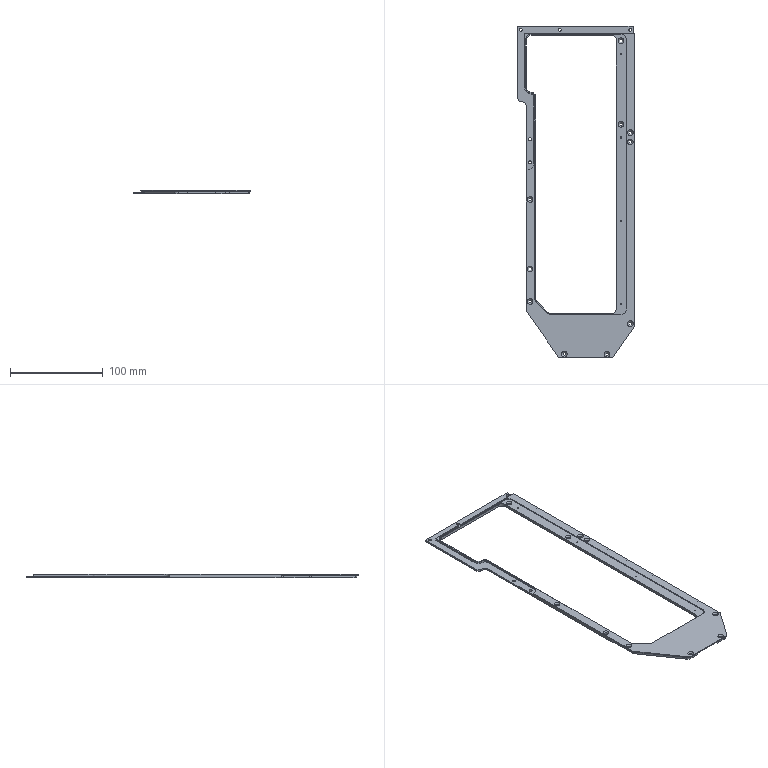NC program | NX | posted with a generic post | part box 127 x 358 x 4 mm
Whole program:
N10 G17 G21 G94 G90
(SPOT_DRILL , TOOL : CHAMFER_D8-90DEG)
N12 T01 M6
N14 G53
N16 G17 G0 G90 X153.952 Y-40.61 S2500 M3
N18 G43 Z20. H1
N20 G94 G82 G98 Z-2.6 F250. P200 R3.
N22 X103.952 Y-30.61
N24 X48.952
N26 X-6.048
N28 X-61.048
N30 X-111.048
N32 X-101. Y3.5
N34 X-111.048 Y28.911
N36 X-61.048
N38 X-6.048
N40 X48.952
N42 X103.952
N44 X119. Y3.5
N46 X153.952 Y28.911
N48 G80
N50 G0 X153.952 Y28.911 Z20.
N52 M5
(SPOT_DRILL_COPY , TOOL : DRILL_D5.3-62-92)
N54 T02 M6
N56 G53
N58 G17 G0 G90 X153.952 Y-40.61 S3000 M3
N60 G43 Z20. H2
N62 G94 G82 G98 Z-6.5 F200. P200 R3.
N64 X103.952 Y-30.61
N66 X48.952
N68 X-6.048
N70 X-61.048
N72 X-111.048
N74 X-101. Y3.5
N76 X-111.048 Y28.911
N78 X-61.048
N80 X-6.048
N82 X48.952
N84 X103.952
N86 X119. Y3.5
N88 X153.952 Y28.911
N90 G80
N92 G0 X153.952 Y28.911 Z20.
N94 M5
(SPOT_DRILL_1 , TOOL : CHAMFER_D8-90DEG)
N96 T01 M6
N98 G53
N100 G17 G0 G90 X175. Y-59.5 S2500 M3
N102 G43 Z20. H1
N104 G94 G82 G98 Z-1.6 F250. P200 R3.
N106 Y-17.5
N108 Y58.5
N110 X163. Y48.5
N112 X73.
N114 X64. Y58.5
N116 X54.
N118 X57. Y-49.5
N120 X32.
N122 X-8.
N124 X-83.
N126 X-118.
N128 X-175. Y-12.5
N130 Y33.5
N132 X-142. Y58.5
N134 G80
N136 G0 X-142. Y58.5 Z20.
N138 M5
(SPOT_DRILL_1_COPY , TOOL : DRILL_D3.2-42-71)
N140 T06 M6
N142 G53
N144 G17 G0 G90 X175. Y-59.5 S3000 M3
N146 G43 Z20. H6
N148 G94 G82 G98 Z-6. F200. P200 R3.
N150 Y-17.5
N152 Y58.5
N154 X163. Y48.5
N156 X73.
N158 X64. Y58.5
N160 X54.
N162 X57. Y-49.5
N164 X32.
N166 X-8.
N168 X-83.
N170 X-118.
N172 X-175. Y-12.5
N174 Y33.5
N176 X-142. Y58.5
N178 G80
N180 G0 X-142. Y58.5 Z20.
N182 M5
(PLANAR_MILL_9 , TOOL : D6-18-D6-50-3T-ROUGH)
N184 T03 M6
N186 G53
N188 G17 G0 G90 X-102.008 Y1.865 S3500 M3
N190 G43 Z20. H3
N192 Z1.
N194 G94 G1 X-101.965 Y1.829 Z0.997 F1500.
N196 X-101.339 Y1.6 Z0.962
N198 X-100.661 Z0.927
N200 X-100.035 Y1.829 Z0.892
N202 X-99.524 Y2.256 Z0.857
N204 X-99.185 Y2.844 Z0.821
N206 X-99.078 Y3.67 Z0.778
N208 X-99.329 Y4.465 Z0.734
N210 X-99.891 Y5.08 Z0.69
N212 X-100.661 Y5.4 Z0.646
N214 X-101.339 Z0.611
N216 X-102.109 Y5.08 Z0.567
N218 X-102.671 Y4.465 Z0.524
N220 X-102.922 Y3.67 Z0.48
N222 X-102.815 Y2.844 Z0.436
N224 X-102.476 Y2.256 Z0.401
N226 X-101.965 Y1.829 Z0.366
N228 X-101.339 Y1.6 Z0.331
N230 X-100.661 Z0.295
N232 X-100.035 Y1.829 Z0.26
N234 X-99.524 Y2.256 Z0.225
N236 X-99.185 Y2.844 Z0.19
N238 X-99.078 Y3.67 Z0.146
N240 X-99.329 Y4.465 Z0.103
N242 X-99.891 Y5.08 Z0.059
N244 X-100.661 Y5.4 Z0.015
N246 X-101.339 Z-0.02
N248 X-102.109 Y5.08 Z-0.064
N250 X-102.671 Y4.465 Z-0.108
N252 X-102.922 Y3.67 Z-0.151
N254 X-102.815 Y2.844 Z-0.195
N256 X-102.476 Y2.256 Z-0.231
N258 X-101.965 Y1.829 Z-0.266
N260 X-101.339 Y1.6 Z-0.3
N262 X-100.661 Z-0.336
N264 X-100.035 Y1.829 Z-0.371
N266 X-99.524 Y2.256 Z-0.406
N268 X-99.185 Y2.844 Z-0.441
N270 X-99.078 Y3.67 Z-0.485
N272 X-99.329 Y4.465 Z-0.529
N274 X-99.891 Y5.08 Z-0.572
N276 X-100.661 Y5.4 Z-0.616
N278 X-101.339 Z-0.652
N280 X-102.109 Y5.08 Z-0.695
N282 X-102.671 Y4.465 Z-0.739
N284 X-102.922 Y3.67 Z-0.783
N286 X-102.815 Y2.844 Z-0.826
N288 X-102.476 Y2.256 Z-0.862
N290 X-101.965 Y1.829 Z-0.897
N292 X-101.339 Y1.6 Z-0.932
N294 X-100.661 Z-0.967
N296 X-100.035 Y1.829 Z-1.002
N298 X-99.524 Y2.256 Z-1.037
N300 X-99.185 Y2.844 Z-1.073
N302 X-99.078 Y3.67 Z-1.116
N304 X-99.329 Y4.465 Z-1.16
N306 X-99.891 Y5.08 Z-1.204
N308 X-100.661 Y5.4 Z-1.247
N310 X-101.339 Z-1.283
N312 X-102.109 Y5.08 Z-1.327
N314 X-102.671 Y4.465 Z-1.37
N316 X-102.922 Y3.67 Z-1.414
N318 X-102.815 Y2.844 Z-1.458
N320 X-102.476 Y2.256 Z-1.493
N322 X-101.965 Y1.829 Z-1.528
N324 X-101.339 Y1.6 Z-1.563
N326 X-100.661 Z-1.599
N328 X-100.035 Y1.829 Z-1.634
N330 X-99.524 Y2.256 Z-1.668
N332 X-99.185 Y2.844 Z-1.704
N334 X-99.078 Y3.67 Z-1.748
N336 X-99.329 Y4.465 Z-1.791
N338 X-99.891 Y5.08 Z-1.835
N340 X-100.661 Y5.4 Z-1.879
N342 X-101.339 Z-1.914
N344 X-102.109 Y5.08 Z-1.958
N346 X-102.671 Y4.465 Z-2.002
N348 X-102.922 Y3.67 Z-2.045
N350 X-102.815 Y2.844 Z-2.089
N352 X-102.476 Y2.256 Z-2.125
N354 X-101.965 Y1.829 Z-2.159
N356 X-101.339 Y1.6 Z-2.194
N358 X-100.661 Z-2.23
N360 X-100.035 Y1.829 Z-2.265
N362 X-99.524 Y2.256 Z-2.3
N364 X-99.185 Y2.844 Z-2.335
N366 X-99.078 Y3.67 Z-2.379
N368 X-99.329 Y4.465 Z-2.423
N370 X-99.891 Y5.08 Z-2.466
N372 X-100.661 Y5.4 Z-2.51
N374 X-101.339 Z-2.546
N376 X-102.109 Y5.08 Z-2.589
N378 X-102.671 Y4.465 Z-2.633
N380 X-102.922 Y3.67 Z-2.677
N382 X-102.815 Y2.844 Z-2.72
N384 X-102.476 Y2.256 Z-2.756
N386 X-101.965 Y1.829 Z-2.791
N388 X-101.339 Y1.6 Z-2.826
N390 X-100.661 Z-2.861
N392 X-100.035 Y1.829 Z-2.896
N394 X-99.524 Y2.256 Z-2.931
N396 X-99.185 Y2.844 Z-2.967
N398 X-99.078 Y3.67 Z-3.01
N400 X-99.329 Y4.465 Z-3.054
N402 X-99.891 Y5.08 Z-3.098
N404 X-100.661 Y5.4 Z-3.141
N406 X-101.339 Z-3.177
N408 X-102.109 Y5.08 Z-3.221
N410 X-102.671 Y4.465 Z-3.264
N412 X-102.922 Y3.67 Z-3.308
N414 X-102.815 Y2.844 Z-3.352
N416 X-102.476 Y2.256 Z-3.387
N418 X-101.965 Y1.829 Z-3.422
N420 X-101.339 Y1.6 Z-3.457
N422 X-100.661 Z-3.493
N424 X-100.035 Y1.829 Z-3.527
N426 X-99.524 Y2.256 Z-3.562
N428 X-99.185 Y2.844 Z-3.598
N430 X-99.078 Y3.67 Z-3.642
N432 X-99.329 Y4.465 Z-3.685
N434 X-99.891 Y5.08 Z-3.729
N436 X-100.661 Y5.4 Z-3.773
N438 X-101.339 Z-3.808
N440 X-102.109 Y5.08 Z-3.852
N442 X-102.671 Y4.465 Z-3.896
N444 X-102.922 Y3.67 Z-3.939
N446 X-102.815 Y2.844 Z-3.983
N448 X-102.476 Y2.256 Z-4.018
N450 X-101.965 Y1.829 Z-4.053
N452 X-101.339 Y1.6 Z-4.088
N454 X-100.661 Z-4.124
N456 X-100.035 Y1.829 Z-4.159
N458 X-99.524 Y2.256 Z-4.194
N460 X-99.185 Y2.844 Z-4.229
N462 X-99.078 Y3.67 Z-4.273
N464 X-99.329 Y4.465 Z-4.317
N466 X-99.891 Y5.08 Z-4.36
N468 X-100.661 Y5.4 Z-4.404
N470 X-101.339 Z-4.44
N472 X-102.109 Y5.08 Z-4.483
N474 X-102.671 Y4.465 Z-4.527
N476 X-102.922 Y3.67 Z-4.571
N478 X-102.815 Y2.844 Z-4.614
N480 X-102.476 Y2.256 Z-4.65
N482 X-101.965 Y1.829 Z-4.685
N484 X-101.339 Y1.6 Z-4.72
N486 X-100.661 Z-4.755
N488 X-100.035 Y1.829 Z-4.79
N490 X-99.524 Y2.256 Z-4.825
N492 X-99.185 Y2.844 Z-4.861
N494 X-99.078 Y3.67 Z-4.904
N496 X-99.329 Y4.465 Z-4.948
N498 X-99.891 Y5.08 Z-4.992
N500 X-100.661 Y5.4 Z-5.035
N502 X-101.339 Z-5.071
N504 X-102.109 Y5.08 Z-5.114
N506 X-102.671 Y4.465 Z-5.158
N508 X-102.922 Y3.67 Z-5.202
N510 X-102.815 Y2.844 Z-5.246
N512 X-102.476 Y2.256 Z-5.281
N514 X-101.965 Y1.829 Z-5.316
N516 X-101.339 Y1.6 Z-5.351
N518 X-100.661 Z-5.386
N520 X-100.035 Y1.829 Z-5.421
N522 X-99.524 Y2.256 Z-5.456
N524 X-99.185 Y2.844 Z-5.492
N526 X-99.078 Y3.67 Z-5.536
N528 X-99.329 Y4.465 Z-5.579
N530 X-99.891 Y5.08 Z-5.623
N532 X-100.661 Y5.4 Z-5.667
N534 X-101.339 Z-5.702
N536 X-102.109 Y5.08 Z-5.746
N538 X-102.671 Y4.465 Z-5.789
N540 X-102.922 Y3.67 Z-5.833
N542 X-102.815 Y2.844 Z-5.877
N544 X-102.476 Y2.256 Z-5.912
N546 X-101.965 Y1.829 Z-5.947
N548 X-101.339 Y1.6 Z-5.982
N550 X-101. Z-6.
N552 G3 X-99.1 Y3.5 R1.9
N554 X-101. Y1.6 R-1.9
N556 G1 Z-5.
N558 G0 Z20.
N560 X117.992 Y1.865
N562 Z1.
N564 G1 X118.035 Y1.829 Z0.997
N566 X118.661 Y1.6 Z0.962
N568 X119.339 Z0.927
N570 X119.965 Y1.829 Z0.892
N572 X120.476 Y2.256 Z0.857
N574 X120.815 Y2.844 Z0.821
N576 X120.922 Y3.67 Z0.778
N578 X120.671 Y4.465 Z0.734
N580 X120.109 Y5.08 Z0.69
N582 X119.339 Y5.4 Z0.646
N584 X118.661 Z0.611
N586 X117.891 Y5.08 Z0.567
N588 X117.329 Y4.465 Z0.524
N590 X117.078 Y3.67 Z0.48
N592 X117.185 Y2.844 Z0.436
N594 X117.524 Y2.256 Z0.401
N596 X118.035 Y1.829 Z0.366
N598 X118.661 Y1.6 Z0.331
N600 X119.339 Z0.295
N602 X119.965 Y1.829 Z0.26
N604 X120.476 Y2.256 Z0.225
N606 X120.815 Y2.844 Z0.19
N608 X120.922 Y3.67 Z0.146
N610 X120.671 Y4.465 Z0.103
N612 X120.109 Y5.08 Z0.059
N614 X119.339 Y5.4 Z0.015
N616 X118.661 Z-0.02
N618 X117.891 Y5.08 Z-0.064
N620 X117.329 Y4.465 Z-0.108
N622 X117.078 Y3.67 Z-0.151
N624 X117.185 Y2.844 Z-0.195
N626 X117.524 Y2.256 Z-0.231
N628 X118.035 Y1.829 Z-0.266
N630 X118.661 Y1.6 Z-0.3
N632 X119.339 Z-0.336
N634 X119.965 Y1.829 Z-0.371
N636 X120.476 Y2.256 Z-0.406
N638 X120.815 Y2.844 Z-0.441
N640 X120.922 Y3.67 Z-0.485
N642 X120.671 Y4.465 Z-0.529
N644 X120.109 Y5.08 Z-0.572
N646 X119.339 Y5.4 Z-0.616
N648 X118.661 Z-0.652
N650 X117.891 Y5.08 Z-0.695
N652 X117.329 Y4.465 Z-0.739
N654 X117.078 Y3.67 Z-0.783
N656 X117.185 Y2.844 Z-0.826
N658 X117.524 Y2.256 Z-0.862
N660 X118.035 Y1.829 Z-0.897
N662 X118.661 Y1.6 Z-0.932
N664 X119.339 Z-0.967
N666 X119.965 Y1.829 Z-1.002
N668 X120.476 Y2.256 Z-1.037
N670 X120.815 Y2.844 Z-1.073
N672 X120.922 Y3.67 Z-1.116
N674 X120.671 Y4.465 Z-1.16
N676 X120.109 Y5.08 Z-1.204
N678 X119.339 Y5.4 Z-1.247
N680 X118.661 Z-1.283
N682 X117.891 Y5.08 Z-1.327
N684 X117.329 Y4.465 Z-1.37
N686 X117.078 Y3.67 Z-1.414
N688 X117.185 Y2.844 Z-1.458
N690 X117.524 Y2.256 Z-1.493
N692 X118.035 Y1.829 Z-1.528
N694 X118.661 Y1.6 Z-1.563
N696 X119.339 Z-1.599
N698 X119.965 Y1.829 Z-1.634
N700 X120.476 Y2.256 Z-1.668
N702 X120.815 Y2.844 Z-1.704
N704 X120.922 Y3.67 Z-1.748
N706 X120.671 Y4.465 Z-1.791
N708 X120.109 Y5.08 Z-1.835
N710 X119.339 Y5.4 Z-1.879
N712 X118.661 Z-1.914
N714 X117.891 Y5.08 Z-1.958
N716 X117.329 Y4.465 Z-2.002
N718 X117.078 Y3.67 Z-2.045
N720 X117.185 Y2.844 Z-2.089
N722 X117.524 Y2.256 Z-2.125
N724 X118.035 Y1.829 Z-2.159
N726 X118.661 Y1.6 Z-2.194
N728 X119.339 Z-2.23
N730 X119.965 Y1.829 Z-2.265
N732 X120.476 Y2.256 Z-2.3
N734 X120.815 Y2.844 Z-2.335
N736 X120.922 Y3.67 Z-2.379
N738 X120.671 Y4.465 Z-2.423
N740 X120.109 Y5.08 Z-2.466
N742 X119.339 Y5.4 Z-2.51
N744 X118.661 Z-2.546
N746 X117.891 Y5.08 Z-2.589
N748 X117.329 Y4.465 Z-2.633
N750 X117.078 Y3.67 Z-2.677
N752 X117.185 Y2.844 Z-2.72
N754 X117.524 Y2.256 Z-2.756
N756 X118.035 Y1.829 Z-2.791
N758 X118.661 Y1.6 Z-2.826
N760 X119.339 Z-2.861
N762 X119.965 Y1.829 Z-2.896
N764 X120.476 Y2.256 Z-2.931
N766 X120.815 Y2.844 Z-2.967
N768 X120.922 Y3.67 Z-3.01
N770 X120.671 Y4.465 Z-3.054
N772 X120.109 Y5.08 Z-3.098
N774 X119.339 Y5.4 Z-3.141
N776 X118.661 Z-3.177
N778 X117.891 Y5.08 Z-3.221
N780 X117.329 Y4.465 Z-3.264
N782 X117.078 Y3.67 Z-3.308
N784 X117.185 Y2.844 Z-3.352
N786 X117.524 Y2.256 Z-3.387
N788 X118.035 Y1.829 Z-3.422
N790 X118.661 Y1.6 Z-3.457
N792 X119.339 Z-3.493
N794 X119.965 Y1.829 Z-3.527
N796 X120.476 Y2.256 Z-3.562
N798 X120.815 Y2.844 Z-3.598
N800 X120.922 Y3.67 Z-3.642
N802 X120.671 Y4.465 Z-3.685
N804 X120.109 Y5.08 Z-3.729
N806 X119.339 Y5.4 Z-3.773
N808 X118.661 Z-3.808
N810 X117.891 Y5.08 Z-3.852
N812 X117.329 Y4.465 Z-3.896
N814 X117.078 Y3.67 Z-3.939
N816 X117.185 Y2.844 Z-3.983
N818 X117.524 Y2.256 Z-4.018
N820 X118.035 Y1.829 Z-4.053
N822 X118.661 Y1.6 Z-4.088
N824 X119.339 Z-4.124
N826 X119.965 Y1.829 Z-4.159
N828 X120.476 Y2.256 Z-4.194
N830 X120.815 Y2.844 Z-4.229
N832 X120.922 Y3.67 Z-4.273
N834 X120.671 Y4.465 Z-4.317
N836 X120.109 Y5.08 Z-4.36
N838 X119.339 Y5.4 Z-4.404
N840 X118.661 Z-4.44
N842 X117.891 Y5.08 Z-4.483
N844 X117.329 Y4.465 Z-4.527
N846 X117.078 Y3.67 Z-4.571
N848 X117.185 Y2.844 Z-4.614
N850 X117.524 Y2.256 Z-4.65
N852 X118.035 Y1.829 Z-4.685
N854 X118.661 Y1.6 Z-4.72
N856 X119.339 Z-4.755
N858 X119.965 Y1.829 Z-4.79
N860 X120.476 Y2.256 Z-4.825
N862 X120.815 Y2.844 Z-4.861
N864 X120.922 Y3.67 Z-4.904
N866 X120.671 Y4.465 Z-4.948
N868 X120.109 Y5.08 Z-4.992
N870 X119.339 Y5.4 Z-5.035
N872 X118.661 Z-5.071
N874 X117.891 Y5.08 Z-5.114
N876 X117.329 Y4.465 Z-5.158
N878 X117.078 Y3.67 Z-5.202
N880 X117.185 Y2.844 Z-5.246
N882 X117.524 Y2.256 Z-5.281
N884 X118.035 Y1.829 Z-5.316
N886 X118.661 Y1.6 Z-5.351
N888 X119.339 Z-5.386
N890 X119.965 Y1.829 Z-5.421
N892 X120.476 Y2.256 Z-5.456
N894 X120.815 Y2.844 Z-5.492
N896 X120.922 Y3.67 Z-5.536
N898 X120.671 Y4.465 Z-5.579
N900 X120.109 Y5.08 Z-5.623
N902 X119.339 Y5.4 Z-5.667
N904 X118.661 Z-5.702
N906 X117.891 Y5.08 Z-5.746
N908 X117.329 Y4.465 Z-5.789
N910 X117.078 Y3.67 Z-5.833
N912 X117.185 Y2.844 Z-5.877
N914 X117.524 Y2.256 Z-5.912
N916 X118.035 Y1.829 Z-5.947
N918 X118.661 Y1.6 Z-5.982
N920 X119. Z-6.
N922 G3 X120.9 Y3.5 R1.9
N924 X119. Y1.6 R-1.9
N926 G1 Z-5.
N928 G0 Z20.
(FLOOR_FACING , TOOL : D6-18-D6-50-3T-ROUGH)
N930 X-183.9 Y8.741
N932 Z2.233
N934 G1 Z-0.767
N936 X-177.9
N938 G3 X-176.4 Y10.241 R1.5
N940 G1 Y22.4
N942 X-165.9
N944 Y31.5
N946 G2 X-164. Y33.4 R1.9
N948 G1 X-132.5
N950 Y-12.4
N952 X-164.
N954 G2 X-165.9 Y-10.5 R1.9
N956 G1 Y-1.4
N958 X-176.4
N960 Y10.241
N962 X-171.9
N964 Y17.9
N966 X-165.9
N968 G3 X-161.4 Y22.4 R4.5
N970 G1 Y28.9
N972 X-137.
N974 Y-7.9
N976 X-161.4
N978 Y-1.4
N980 G3 X-165.9 Y3.1 R4.5
N982 G1 X-171.9
N984 Y10.241
N986 X-167.4
N988 Y13.4
N990 X-165.9
N992 G3 X-156.9 Y22.4 R9.
N994 G1 Y24.4
N996 X-141.5
N998 Y-3.4
N1000 X-156.9
N1002 Y-1.4
N1004 G3 X-165.9 Y7.6 R9.
N1006 G1 X-167.4
N1008 Y10.241
N1010 X-159.525 Y10.5
N1012 G3 X-152.634 Y19.9 R13.5
N1014 G1 X-146.
N1016 Y1.1
N1018 X-152.634
N1020 G3 X-159.525 Y10.5 R13.5
N1022 G1 X-152.395
N1024 G3 X-150.5 Y13.081 R18.
N1026 G1 X-149.699 Y16.406
N1028 X-150.5 Y13.081
N1030 Y7.919
N1032 X-149.699 Y4.594
N1034 X-150.5 Y7.919
N1036 G3 X-152.395 Y10.5 R18.
N1038 X-151.755 Y11.268 R18.
N1040 X-152.006 Y13.375 R1.5
N1042 G1 Z2.233
N1044 G0 Z20.
N1046 X-183.9 Y8.741
N1048 Z1.467
N1050 G1 Z-1.533
N1052 X-177.9
N1054 G3 X-176.4 Y10.241 R1.5
N1056 G1 Y22.4
N1058 X-165.9
N1060 Y31.5
N1062 G2 X-164. Y33.4 R1.9
N1064 G1 X-132.5
N1066 Y-12.4
N1068 X-164.
N1070 G2 X-165.9 Y-10.5 R1.9
N1072 G1 Y-1.4
N1074 X-176.4
N1076 Y10.241
N1078 X-171.9
N1080 Y17.9
N1082 X-165.9
N1084 G3 X-161.4 Y22.4 R4.5
N1086 G1 Y28.9
N1088 X-137.
N1090 Y-7.9
N1092 X-161.4
N1094 Y-1.4
N1096 G3 X-165.9 Y3.1 R4.5
N1098 G1 X-171.9
N1100 Y10.241
N1102 X-167.4
N1104 Y13.4
N1106 X-165.9
N1108 G3 X-156.9 Y22.4 R9.
N1110 G1 Y24.4
N1112 X-141.5
N1114 Y-3.4
N1116 X-156.9
N1118 Y-1.4
N1120 G3 X-165.9 Y7.6 R9.
N1122 G1 X-167.4
N1124 Y10.241
N1126 X-159.525 Y10.5
N1128 G3 X-152.634 Y19.9 R13.5
N1130 G1 X-146.
N1132 Y1.1
N1134 X-152.634
N1136 G3 X-159.525 Y10.5 R13.5
N1138 G1 X-152.395
N1140 G3 X-150.5 Y13.081 R18.
N1142 G1 X-149.699 Y16.406
N1144 X-150.5 Y13.081
N1146 Y7.919
N1148 X-149.699 Y4.594
N1150 X-150.5 Y7.919
N1152 G3 X-152.395 Y10.5 R18.
N1154 X-151.755 Y11.268 R18.
N1156 X-152.006 Y13.375 R1.5
N1158 G1 Z1.467
N1160 G0 Z20.
N1162 X-183.9 Y8.741
N1164 Z0.7
N1166 G1 Z-2.3
N1168 X-177.9
N1170 G3 X-176.4 Y10.241 R1.5
N1172 G1 Y22.4
N1174 X-165.9
N1176 Y31.5
N1178 G2 X-164. Y33.4 R1.9
N1180 G1 X-132.5
N1182 Y-12.4
N1184 X-164.
N1186 G2 X-165.9 Y-10.5 R1.9
N1188 G1 Y-1.4
N1190 X-176.4
N1192 Y10.241
N1194 X-171.9
N1196 Y17.9
N1198 X-165.9
N1200 G3 X-161.4 Y22.4 R4.5
N1202 G1 Y28.9
N1204 X-137.
N1206 Y-7.9
N1208 X-161.4
N1210 Y-1.4
N1212 G3 X-165.9 Y3.1 R4.5
N1214 G1 X-171.9
N1216 Y10.241
N1218 X-167.4
N1220 Y13.4
N1222 X-165.9
N1224 G3 X-156.9 Y22.4 R9.
N1226 G1 Y24.4
N1228 X-141.5
N1230 Y-3.4
N1232 X-156.9
N1234 Y-1.4
N1236 G3 X-165.9 Y7.6 R9.
N1238 G1 X-167.4
N1240 Y10.241
N1242 X-159.525 Y10.5
N1244 G3 X-152.634 Y19.9 R13.5
N1246 G1 X-146.
N1248 Y1.1
N1250 X-152.634
N1252 G3 X-159.525 Y10.5 R13.5
N1254 G1 X-152.395
N1256 G3 X-150.5 Y13.081 R18.
N1258 G1 X-149.699 Y16.406
N1260 X-150.5 Y13.081
N1262 Y7.919
N1264 X-149.699 Y4.594
N1266 X-150.5 Y7.919
N1268 G3 X-152.395 Y10.5 R18.
N1270 X-151.755 Y11.268 R18.
N1272 X-152.006 Y13.375 R1.5
N1274 G1 Z0.7
N1276 G0 Z20.
(PLANAR_MILL , TOOL : D6-18-D6-50-3T-ROUGH)
N1278 X-183.9 Y-1.3
N1280 Z0.6
N1282 G1 Z-2.4
N1284 X-177.9
N1286 X-169.
N1288 G2 X-165.8 Y-4.5 R3.2
N1290 G1 Y-10.5
N1292 G3 X-164. Y-12.3 R1.8
N1294 G1 X-134.2
N1296 Y33.3
N1298 X-164.
N1300 G3 X-165.8 Y31.5 R1.8
N1302 G1 Y25.5
N1304 G2 X-169. Y22.3 R3.2
N1306 G1 X-177.9
N1308 X-183.9
N1310 Z0.6
N1312 G0 Z20.
(PLANAR_MILL_1_COPY_1 , TOOL : D6-18-D6-50-3T-ROUGH)
N1314 X185. Y-66.6
N1316 Z2.14
N1318 G1 Z-0.86
N1320 X179.
N1322 X102.5
N1324 G2 X94.4 Y-58.5 R8.1
N1326 G3 X92.5 Y-56.6 R1.9
N1328 G1 X-127.869
N1330 G2 X-130.795 Y-55.678 R5.1
N1332 G1 X-179.925 Y-21.276
N1334 G2 X-182.1 Y-17.098 R5.1
N1336 G1 Y37.952
N1338 G2 X-179.925 Y42.129 R5.1
N1340 G1 X-146.295 Y65.678
N1342 G2 X-143.369 Y66.6 R5.1
N1344 G1 X181.9
N1346 X187.9
N1348 Z2.14
N1350 G0 Z20.
N1352 X185. Y-66.6
N1354 Z1.28
N1356 G1 Z-1.72
N1358 X179.
N1360 X102.5
N1362 G2 X94.4 Y-58.5 R8.1
N1364 G3 X92.5 Y-56.6 R1.9
N1366 G1 X-127.869
N1368 G2 X-130.795 Y-55.678 R5.1
N1370 G1 X-179.925 Y-21.276
N1372 G2 X-182.1 Y-17.098 R5.1
N1374 G1 Y37.952
N1376 G2 X-179.925 Y42.129 R5.1
N1378 G1 X-146.295 Y65.678
N1380 G2 X-143.369 Y66.6 R5.1
N1382 G1 X181.9
N1384 X187.9
N1386 Z1.28
N1388 G0 Z20.
N1390 X185. Y-66.6
N1392 Z0.42
N1394 G1 Z-2.58
N1396 X179.
N1398 X102.5
N1400 G2 X94.4 Y-58.5 R8.1
N1402 G3 X92.5 Y-56.6 R1.9
N1404 G1 X-127.869
N1406 G2 X-130.795 Y-55.678 R5.1
N1408 G1 X-179.925 Y-21.276
N1410 G2 X-182.1 Y-17.098 R5.1
N1412 G1 Y37.952
N1414 G2 X-179.925 Y42.129 R5.1
N1416 G1 X-146.295 Y65.678
N1418 G2 X-143.369 Y66.6 R5.1
N1420 G1 X181.9
N1422 X187.9
N1424 Z0.42
N1426 G0 Z20.
N1428 X185. Y-66.6
N1430 Z-0.44
N1432 G1 Z-3.44
N1434 X179.
N1436 X102.5
N1438 G2 X94.4 Y-58.5 R8.1
N1440 G3 X92.5 Y-56.6 R1.9
N1442 G1 X-127.869
N1444 G2 X-130.795 Y-55.678 R5.1
N1446 G1 X-179.925 Y-21.276
N1448 G2 X-182.1 Y-17.098 R5.1
N1450 G1 Y37.952
N1452 G2 X-179.925 Y42.129 R5.1
N1454 G1 X-146.295 Y65.678
N1456 G2 X-143.369 Y66.6 R5.1
N1458 G1 X181.9
N1460 X187.9
N1462 Z-0.44
N1464 G0 Z20.
N1466 X185. Y-66.6
N1468 Z-1.3
N1470 G1 Z-4.3
N1472 X179.
N1474 X102.5
N1476 G2 X94.4 Y-58.5 R8.1
N1478 G3 X92.5 Y-56.6 R1.9
N1480 G1 X-127.869
N1482 G2 X-130.795 Y-55.678 R5.1
N1484 G1 X-179.925 Y-21.276
N1486 G2 X-182.1 Y-17.098 R5.1
N1488 G1 Y37.952
N1490 G2 X-179.925 Y42.129 R5.1
N1492 G1 X-146.295 Y65.678
N1494 G2 X-143.369 Y66.6 R5.1
N1496 G1 X181.9
N1498 X187.9
N1500 Z-1.3
N1502 G0 Z20.
(PLANAR_MILL_1_COPY_1_COPY , TOOL : D6-18-D6-50-3T-ROUGH)
N1504 X182.1 Y67.5
N1506 Z2.14
N1508 G1 Z-0.86
N1510 Y61.5
N1512 Y-63.5
N1514 Y-69.5
N1516 Z2.14
N1518 G0 Z20.
N1520 Y67.5
N1522 Z1.28
N1524 G1 Z-1.72
N1526 Y61.5
N1528 Y-63.5
N1530 Y-69.5
N1532 Z1.28
N1534 G0 Z20.
N1536 Y67.5
N1538 Z0.42
N1540 G1 Z-2.58
N1542 Y61.5
N1544 Y-63.5
N1546 Y-69.5
N1548 Z0.42
N1550 G0 Z20.
N1552 Y67.5
N1554 Z-0.44
N1556 G1 Z-3.44
N1558 Y61.5
N1560 Y-63.5
N1562 Y-69.5
N1564 Z-0.44
N1566 G0 Z20.
N1568 Y67.5
N1570 Z-1.3
N1572 G1 Z-4.3
N1574 Y61.5
N1576 Y-63.5
N1578 Y-69.5
N1580 Z-1.3
N1582 G0 Z20.
(PLANAR_MILL_1 , TOOL : D6-18-D6-50-3T-ROUGH)
N1584 X-93.06 Y-59.58
N1586 Z2.
N1588 G1 Z-1.
N1590 X-97.86 Y-55.98
N1592 G3 X-99. Y-55.6 R1.9
N1594 G1 X-126.434
N1596 G2 X-131.08 Y-54.135 R8.1
N1598 G1 X-177.546 Y-21.599
N1600 G2 X-181. Y-14.964 R8.1
N1602 G1 Y35.817
N1604 G2 X-177.546 Y42.452 R8.1
N1606 G1 X-148.008 Y63.135
N1608 G2 X-143.362 Y64.6 R8.1
N1610 G1 X179.
N1612 X185.
N1614 Z2.
N1616 G0 Z20.
N1618 X-93.06 Y-59.58
N1620 Z1.
N1622 G1 Z-2.
N1624 X-97.86 Y-55.98
N1626 G3 X-99. Y-55.6 R1.9
N1628 G1 X-126.434
N1630 G2 X-131.08 Y-54.135 R8.1
N1632 G1 X-177.546 Y-21.599
N1634 G2 X-181. Y-14.964 R8.1
N1636 G1 Y35.817
N1638 G2 X-177.546 Y42.452 R8.1
N1640 G1 X-148.008 Y63.135
N1642 G2 X-143.362 Y64.6 R8.1
N1644 G1 X179.
N1646 X185.
N1648 Z1.
N1650 G0 Z20.
N1652 X-93.06 Y-59.58
N1654 Z0.1
N1656 G1 Z-2.9
N1658 X-97.86 Y-55.98
N1660 G3 X-99. Y-55.6 R1.9
N1662 G1 X-126.434
N1664 G2 X-131.08 Y-54.135 R8.1
N1666 G1 X-177.546 Y-21.599
N1668 G2 X-181. Y-14.964 R8.1
N1670 G1 Y35.817
N1672 G2 X-177.546 Y42.452 R8.1
N1674 G1 X-148.008 Y63.135
N1676 G2 X-143.362 Y64.6 R8.1
N1678 G1 X179.
N1680 X185.
N1682 Z0.1
N1684 G0 Z20.
N1686 M5
(PLANAR_MILL_9_COPY , TOOL : D6-18-D6-50-3T-FINISH)
N1688 T04 M6
N1690 G53
N1692 G17 G0 G90 X-101.965 Y3.697 S3500 M3
N1694 G43 Z20. H4
N1696 Z-4.
N1698 G94 G1 Z-6. F500.
N1700 G41 X-102. Y3.5 D4
N1702 Y2.5
N1704 G3 X-101. Y1.5 R1.
N1706 X-99. Y3.5 R2.
N1708 X-101. Y1.5 R-2.
N1710 X-100. Y2.5 R1.
N1712 G40
N1714 G1 X-100.035 Y2.697
N1716 X-101.965
N1718 G41 X-102. Y2.5
N1720 G3 X-101. Y1.5 R1.
N1722 X-99. Y3.5 R2.
N1724 X-101. Y1.5 R-2.
N1726 X-100. Y2.5 R1.
N1728 G1 Y3.499
N1730 G40
N1732 X-100.035 Y3.696
N1734 Z-4.
N1736 G0 Z20.
N1738 X118.035 Y3.697
N1740 Z-4.
N1742 G1 Z-6.
N1744 G41 X118. Y3.5
N1746 Y2.5
N1748 G3 X119. Y1.5 R1.
N1750 X121. Y3.5 R2.
N1752 X119. Y1.5 R-2.
N1754 X120. Y2.5 R1.
N1756 G40
N1758 G1 X119.965 Y2.697
N1760 X118.035
N1762 G41 X118. Y2.5
N1764 G3 X119. Y1.5 R1.
N1766 X121. Y3.5 R2.
N1768 X119. Y1.5 R-2.
N1770 X120. Y2.5 R1.
N1772 G1 Y3.499
N1774 G40
N1776 X119.965 Y3.696
N1778 Z-4.
N1780 G0 Z20.
(FLOOR_FACING_COPY , TOOL : D6-18-D6-50-3T-FINISH)
N1782 X-183.9 Y8.741
N1784 Z0.5
N1786 G1 Z-2.5 F800.
N1788 X-177.9
N1790 G3 X-176.4 Y10.241 R1.5
N1792 G1 Y22.5
N1794 X-166.
N1796 Y31.5
N1798 G2 X-164. Y33.5 R2.
N1800 G1 X-132.5
N1802 Y-12.5
N1804 X-164.
N1806 G2 X-166. Y-10.5 R2.
N1808 G1 Y-1.5
N1810 X-176.4
N1812 Y10.241
N1814 X-171.9
N1816 Y18.
N1818 X-166.
N1820 G3 X-161.5 Y22.5 R4.5
N1822 G1 Y29.
N1824 X-137.
N1826 Y-8.
N1828 X-161.5
N1830 Y-1.5
N1832 G3 X-166. Y3. R4.5
N1834 G1 X-171.9
N1836 Y10.241
N1838 X-167.4
N1840 Y13.5
N1842 X-166.
N1844 G3 X-157. Y22.5 R9.
N1846 G1 Y24.5
N1848 X-141.5
N1850 Y-3.5
N1852 X-157.
N1854 Y-1.5
N1856 G3 X-166. Y7.5 R9.
N1858 G1 X-167.4
N1860 Y10.241
N1862 X-159.815 Y10.5
N1864 G3 X-152.734 Y20. R13.5
N1866 G1 X-146.
N1868 Y1.
N1870 X-152.734
N1872 G3 X-159.815 Y10.5 R13.5
N1874 G1 X-152.584
N1876 G3 X-150.5 Y13.348 R18.
N1878 G1 X-149.717 Y16.595
N1880 X-150.5 Y13.348
N1882 Y7.652
N1884 X-149.717 Y4.405
N1886 X-150.5 Y7.652
N1888 G3 X-152.584 Y10.5 R18.
N1890 X-151.938 Y11.263 R18.
N1892 X-152.173 Y13.372 R1.5
N1894 G1 Z0.5
N1896 G0 Z20.
(PLANAR_MILL_COPY , TOOL : D6-18-D6-50-3T-FINISH)
N1898 X-184.097 Y-1.465
N1900 Z0.5
N1902 G1 Z-2.5
N1904 G41 X-183.9 Y-1.5
N1906 X-177.9
N1908 X-169.
N1910 G2 X-166. Y-4.5 R3.
N1912 G1 Y-10.5
N1914 G3 X-164. Y-12.5 R2.
N1916 G1 X-134.
N1918 Y33.5
N1920 X-164.
N1922 G3 X-166. Y31.5 R2.
N1924 G1 Y25.5
N1926 G2 X-169. Y22.5 R3.
N1928 G1 X-177.9
N1930 X-183.9
N1932 G40
N1934 X-184.097 Y22.465
N1936 Z0.5
N1938 G0 Z20.
(PLANAR_MILL_1_COPY_1_COPY_1 , TOOL : D6-18-D6-50-3T-FINISH)
N1940 X185.197 Y-66.535
N1942 Z-1.3
N1944 G1 Z-4.3
N1946 G41 X185. Y-66.5
N1948 X179.
N1950 X102.5
N1952 G2 X94.5 Y-58.5 R8.
N1954 G3 X92.5 Y-56.5 R2.
N1956 G1 X-127.869
N1958 G2 X-130.737 Y-55.596 R5.
N1960 G1 X-179.868 Y-21.194
N1962 G2 X-182. Y-17.098 R5.
N1964 G1 Y37.952
N1966 G2 X-179.868 Y42.047 R5.
N1968 G1 X-146.237 Y65.596
N1970 G2 X-143.369 Y66.5 R5.
N1972 G1 X181.9
N1974 X187.9
N1976 G40
N1978 X188.097 Y66.535
N1980 Z-1.3
N1982 G0 Z20.
(PLANAR_MILL_1_COPY_1_COPY_COPY , TOOL : D6-18-D6-50-3T-FINISH)
N1984 X182.035 Y67.697
N1986 Z-1.3
N1988 G1 Z-4.3
N1990 G41 X182. Y67.5
N1992 Y61.5
N1994 Y-63.5
N1996 Y-69.5
N1998 G40
N2000 X182.035 Y-69.697
N2002 Z-1.3
N2004 G0 Z20.
(PLANAR_MILL_1_COPY , TOOL : D6-18-D6-50-3T-FINISH)
N2006 X-92.863 Y-59.646
N2008 Z0.
N2010 G1 Z-3.
N2012 G41 X-93. Y-59.5
N2014 X-97.8 Y-55.9
N2016 G3 X-99. Y-55.5 R2.
N2018 G1 X-126.434
N2020 G2 X-131.022 Y-54.053 R8.
N2022 G1 X-177.489 Y-21.517
N2024 G2 X-180.9 Y-14.964 R8.
N2026 G1 Y35.817
N2028 G2 X-177.489 Y42.37 R8.
N2030 G1 X-147.951 Y63.053
N2032 G2 X-143.362 Y64.5 R8.
N2034 G1 X179.
N2036 X185.
N2038 G40
N2040 X185.197 Y64.535
N2042 Z0.
N2044 G0 Z20.
N2046 M5
(PLANAR_MILL_7 , TOOL : CHAMFER_D3-90DEG)
N2048 T08 M6
N2050 G53
N2052 G17 G0 G90 X-128.703 Y35.865 S3000 M3
N2054 G43 Z20. H8
N2056 Z2.4
N2058 G94 G1 Z-0.6 F1000.
N2060 G41 X-128.9 Y35.9 D8
N2062 X-129.5
N2064 X-131.
N2066 X-164.
N2068 G3 X-168.4 Y31.5 R4.4
N2070 G1 Y25.5
N2072 G2 X-169. Y24.9 R0.6
N2074 G1 X-177.9
N2076 G2 X-178.5 Y25.5 R0.6
N2078 G1 Y35.817
N2080 G2 X-176.112 Y40.405 R5.6
N2082 G1 X-146.574 Y61.087
N2084 G2 X-143.362 Y62.1 R5.6
N2086 G1 X179.
N2088 G2 X179.6 Y61.5 R0.6
N2090 G1 Y-63.5
N2092 G2 X179. Y-64.1 R0.6
N2094 G1 X102.5
N2096 G2 X96.9 Y-58.5 R5.6
N2098 G3 X92.5 Y-54.1 R4.4
N2100 G1 X-96.
N2102 G2 X-96.36 Y-53.98 R0.6
N2104 G3 X-99. Y-53.1 R4.4
N2106 G1 X-126.434
N2108 G2 X-129.646 Y-52.087 R5.6
N2110 G1 X-176.112 Y-19.551
N2112 G2 X-178.5 Y-14.964 R5.6
N2114 G1 Y-4.5
N2116 G2 X-177.9 Y-3.9 R0.6
N2118 G1 X-169.
N2120 G2 X-168.4 Y-4.5 R0.6
N2122 G1 Y-10.5
N2124 G3 X-164. Y-14.9 R4.4
N2126 G1 X-131.
N2128 X-128.9
N2130 G40
N2132 X-128.703 Y-14.865
N2134 Z2.4
N2136 G0 Z20.
(PLANAR_MILL_7_COPY , TOOL : CHAMFER_D3-90DEG)
N2138 X-98.904 Y-55.297
N2140 Z-1.6
N2142 G1 Z-3.6
N2144 G41 X-98.869 Y-55.1
N2146 G3 X-99.869 Y-54.1 R1.
N2148 G1 X-127.869
N2150 G2 X-129.361 Y-53.63 R2.6
N2152 G1 X-178.491 Y-19.228
N2154 G2 X-179.6 Y-17.098 R2.6
N2156 G1 Y37.952
N2158 G2 X-178.491 Y40.081 R2.6
N2160 G1 X-144.861 Y63.63
N2162 G2 X-143.369 Y64.1 R2.6
N2164 G1 X170.9
N2166 G3 X171.9 Y65.1 R1.
N2168 G40
N2170 G1 X171.865 Y65.297
N2172 Z-1.6
N2174 G0 Z20.
(PLANAR_MILL_7_COPY_COPY , TOOL : CHAMFER_D3-90DEG)
N2176 X-101.965 Y0.657
N2178 Z1.
N2180 G1 Z-1.
N2182 G41 X-102. Y0.46
N2184 Y0.3
N2186 G3 X-101. Y-0.7 R1.
N2188 X-96.8 Y3.5 R4.2
N2190 X-101. Y-0.7 R-4.2
N2192 X-100. Y0.3 R1.
N2194 G1 Y0.46
N2196 G40
N2198 X-100.035 Y0.657
N2200 Z1.
N2202 G0 Z20.
N2204 X118.035
N2206 Z1.
N2208 G1 Z-1.
N2210 G41 X118. Y0.46
N2212 Y0.3
N2214 G3 X119. Y-0.7 R1.
N2216 X123.2 Y3.5 R4.2
N2218 X119. Y-0.7 R-4.2
N2220 X120. Y0.3 R1.
N2222 G1 Y0.46
N2224 G40
N2226 X119.965 Y0.657
N2228 Z1.
N2230 G0 Z20.
N2232 M5
N2234 M2